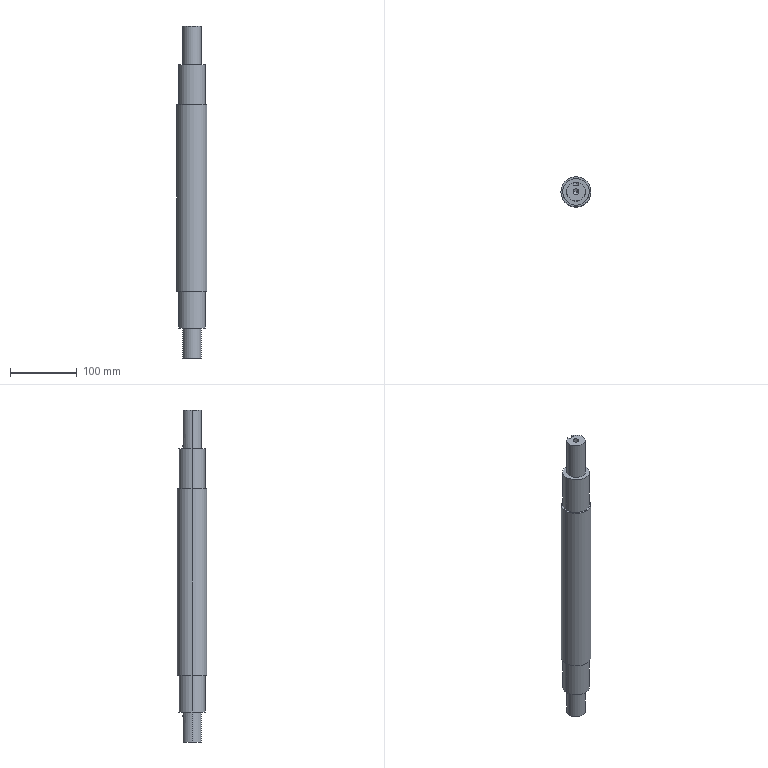Part | STEP file | Produce dryer line heating fan-SIROCCOFAN-3KW-SHAFT | 1 solid | 34 faces | box 45 x 45 x 498 mm | volume 647195 mm3 | cylinder 18 | plane 12 | cone 4 | commonest cylinder face diameters 8 x4 8.5 x4 28 x4 40 x4 45 x2
STEP:
#1=CARTESIAN_POINT('',(4.25,0.,-352.5));
#2=VERTEX_POINT('',#1);
#3=CARTESIAN_POINT('',(-4.25,0.,-352.5));
#4=VERTEX_POINT('',#3);
#5=CARTESIAN_POINT('',(0.,0.,-352.5));
#6=DIRECTION('',(0.,0.,-1.));
#7=DIRECTION('',(-1.,0.,0.));
#8=AXIS2_PLACEMENT_3D('',#5,#6,#7);
#9=CIRCLE('',#8,4.25);
#10=EDGE_CURVE('',#2,#4,#9,.T.);
#11=ORIENTED_EDGE('',*,*,#10,.F.);
#12=CARTESIAN_POINT('',(4.25,0.,-380.));
#13=VERTEX_POINT('',#12);
#14=CARTESIAN_POINT('',(4.25,0.,-380.));
#15=DIRECTION('',(0.,0.,-1.));
#16=VECTOR('',#15,1000.);
#17=LINE('',#14,#16);
#18=EDGE_CURVE('',#2,#13,#17,.T.);
#19=ORIENTED_EDGE('',*,*,#18,.T.);
#20=CARTESIAN_POINT('',(-4.25,0.,-380.));
#21=VERTEX_POINT('',#20);
#22=CARTESIAN_POINT('',(0.,0.,-380.));
#23=DIRECTION('',(0.,0.,-1.));
#24=DIRECTION('',(-1.,0.,0.));
#25=AXIS2_PLACEMENT_3D('',#22,#23,#24);
#26=CIRCLE('',#25,4.25);
#27=EDGE_CURVE('',#13,#21,#26,.T.);
#28=ORIENTED_EDGE('',*,*,#27,.T.);
#29=CARTESIAN_POINT('',(-4.25,0.,-380.));
#30=DIRECTION('',(0.,0.,-1.));
#31=VECTOR('',#30,1000.);
#32=LINE('',#29,#31);
#33=EDGE_CURVE('',#4,#21,#32,.T.);
#34=ORIENTED_EDGE('',*,*,#33,.F.);
#35=EDGE_LOOP('',(#11,#19,#28,#34));
#36=FACE_OUTER_BOUND('',#35,.T.);
#37=CARTESIAN_POINT('',(0.,0.,-380.));
#38=DIRECTION('',(0.,0.,-1.));
#39=DIRECTION('',(-1.,0.,0.));
#40=AXIS2_PLACEMENT_3D('',#37,#38,#39);
#41=CYLINDRICAL_SURFACE('',#40,4.25);
#42=ADVANCED_FACE('',(#36),#41,.F.);
#43=CARTESIAN_POINT('',(0.,0.,-349.946));
#44=VERTEX_POINT('',#43);
#45=CARTESIAN_POINT('',(-4.25,0.,-352.5));
#46=DIRECTION('',(-0.8572,0.,-0.515));
#47=VECTOR('',#46,1000.);
#48=LINE('',#45,#47);
#49=EDGE_CURVE('',#44,#4,#48,.T.);
#50=ORIENTED_EDGE('',*,*,#49,.F.);
#51=CARTESIAN_POINT('',(4.25,0.,-352.5));
#52=DIRECTION('',(0.8572,0.,-0.515));
#53=VECTOR('',#52,1000.);
#54=LINE('',#51,#53);
#55=EDGE_CURVE('',#44,#2,#54,.T.);
#56=ORIENTED_EDGE('',*,*,#55,.T.);
#57=ORIENTED_EDGE('',*,*,#10,.T.);
#58=EDGE_LOOP('',(#50,#56,#57));
#59=FACE_OUTER_BOUND('',#58,.T.);
#60=CARTESIAN_POINT('',(0.,0.,-352.5));
#61=DIRECTION('',(0.,0.,-1.));
#62=DIRECTION('',(-1.,0.,0.));
#63=AXIS2_PLACEMENT_3D('',#60,#61,#62);
#64=CONICAL_SURFACE('',#63,4.25,1.03);
#65=ADVANCED_FACE('',(#59),#64,.F.);
#66=CARTESIAN_POINT('',(-14.,0.,-380.));
#67=VERTEX_POINT('',#66);
#68=CARTESIAN_POINT('',(-4.,13.416,-380.));
#69=VERTEX_POINT('',#68);
#70=CARTESIAN_POINT('',(0.,0.,-380.));
#71=DIRECTION('',(0.,0.,-1.));
#72=DIRECTION('',(-1.,0.,0.));
#73=AXIS2_PLACEMENT_3D('',#70,#71,#72);
#74=CIRCLE('',#73,14.);
#75=EDGE_CURVE('',#67,#69,#74,.T.);
#76=ORIENTED_EDGE('',*,*,#75,.F.);
#77=CARTESIAN_POINT('',(-14.,0.,-335.));
#78=VERTEX_POINT('',#77);
#79=CARTESIAN_POINT('',(-14.,0.,-380.));
#80=DIRECTION('',(0.,0.,1.));
#81=VECTOR('',#80,1000.);
#82=LINE('',#79,#81);
#83=EDGE_CURVE('',#67,#78,#82,.T.);
#84=ORIENTED_EDGE('',*,*,#83,.T.);
#85=CARTESIAN_POINT('',(14.,0.,-335.));
#86=VERTEX_POINT('',#85);
#87=CARTESIAN_POINT('',(0.,0.,-335.));
#88=DIRECTION('',(0.,0.,-1.));
#89=DIRECTION('',(-1.,0.,0.));
#90=AXIS2_PLACEMENT_3D('',#87,#88,#89);
#91=CIRCLE('',#90,14.);
#92=EDGE_CURVE('',#78,#86,#91,.T.);
#93=ORIENTED_EDGE('',*,*,#92,.T.);
#94=CARTESIAN_POINT('',(14.,0.,-380.));
#95=VERTEX_POINT('',#94);
#96=CARTESIAN_POINT('',(14.,0.,-380.));
#97=DIRECTION('',(0.,0.,1.));
#98=VECTOR('',#97,1000.);
#99=LINE('',#96,#98);
#100=EDGE_CURVE('',#95,#86,#99,.T.);
#101=ORIENTED_EDGE('',*,*,#100,.F.);
#102=CARTESIAN_POINT('',(4.,13.416,-380.));
#103=VERTEX_POINT('',#102);
#104=CARTESIAN_POINT('',(0.,0.,-380.));
#105=DIRECTION('',(0.,0.,-1.));
#106=DIRECTION('',(-1.,0.,0.));
#107=AXIS2_PLACEMENT_3D('',#104,#105,#106);
#108=CIRCLE('',#107,14.);
#109=EDGE_CURVE('',#103,#95,#108,.T.);
#110=ORIENTED_EDGE('',*,*,#109,.F.);
#111=CARTESIAN_POINT('',(4.,13.416,-344.));
#112=VERTEX_POINT('',#111);
#113=CARTESIAN_POINT('',(4.,13.416,-380.));
#114=DIRECTION('',(0.,0.,1.));
#115=VECTOR('',#114,1000.);
#116=LINE('',#113,#115);
#117=EDGE_CURVE('',#103,#112,#116,.T.);
#118=ORIENTED_EDGE('',*,*,#117,.T.);
#119=CARTESIAN_POINT('',(0.,14.,-340.));
#120=VERTEX_POINT('',#119);
#121=CARTESIAN_POINT('',(4.,13.416,-344.));
#122=CARTESIAN_POINT('',(4.,13.416,-343.734));
#123=CARTESIAN_POINT('',(3.974,13.424,-343.474));
#124=CARTESIAN_POINT('',(3.871,13.454,-342.961));
#125=CARTESIAN_POINT('',(3.794,13.477,-342.706));
#126=CARTESIAN_POINT('',(3.593,13.531,-342.223));
#127=CARTESIAN_POINT('',(3.47,13.564,-341.994));
#128=CARTESIAN_POINT('',(3.18,13.635,-341.56));
#129=CARTESIAN_POINT('',(3.013,13.673,-341.356));
#130=CARTESIAN_POINT('',(2.646,13.749,-340.989));
#131=CARTESIAN_POINT('',(2.446,13.786,-340.824));
#132=CARTESIAN_POINT('',(2.009,13.857,-340.531));
#133=CARTESIAN_POINT('',(1.779,13.889,-340.408));
#134=CARTESIAN_POINT('',(1.299,13.942,-340.208));
#135=CARTESIAN_POINT('',(1.046,13.963,-340.13));
#136=CARTESIAN_POINT('',(0.5278,13.992,-340.026));
#137=CARTESIAN_POINT('',(0.2656,14.,-340.));
#138=CARTESIAN_POINT('',(0.,14.,-340.));
#139=B_SPLINE_CURVE_WITH_KNOTS('',3,(#121,#122,#123,#124,#125,#126,#127,#128,#129,#130,#131,#132,#133,#134,#135,#136,#137,#138),.UNSPECIFIED.,.F.,.F.,(4,2,2,2,2,2,2,2,4),(0.,0.0007852,0.00157,0.002356,0.003141,0.003926,0.004711,0.005496,0.006282),.UNSPECIFIED.);
#140=EDGE_CURVE('',#112,#120,#139,.T.);
#141=ORIENTED_EDGE('',*,*,#140,.T.);
#142=CARTESIAN_POINT('',(-4.,13.416,-344.));
#143=VERTEX_POINT('',#142);
#144=CARTESIAN_POINT('',(0.,14.,-340.));
#145=CARTESIAN_POINT('',(-0.2656,14.,-340.));
#146=CARTESIAN_POINT('',(-0.5265,13.992,-340.026));
#147=CARTESIAN_POINT('',(-1.039,13.964,-340.129));
#148=CARTESIAN_POINT('',(-1.294,13.942,-340.206));
#149=CARTESIAN_POINT('',(-1.778,13.889,-340.407));
#150=CARTESIAN_POINT('',(-2.007,13.857,-340.53));
#151=CARTESIAN_POINT('',(-2.44,13.787,-340.82));
#152=CARTESIAN_POINT('',(-2.645,13.749,-340.988));
#153=CARTESIAN_POINT('',(-3.011,13.674,-341.354));
#154=CARTESIAN_POINT('',(-3.176,13.636,-341.555));
#155=CARTESIAN_POINT('',(-3.469,13.564,-341.991));
#156=CARTESIAN_POINT('',(-3.592,13.532,-342.221));
#157=CARTESIAN_POINT('',(-3.792,13.477,-342.702));
#158=CARTESIAN_POINT('',(-3.87,13.455,-342.954));
#159=CARTESIAN_POINT('',(-3.974,13.424,-343.472));
#160=CARTESIAN_POINT('',(-4.,13.416,-343.734));
#161=CARTESIAN_POINT('',(-4.,13.416,-344.));
#162=B_SPLINE_CURVE_WITH_KNOTS('',3,(#144,#145,#146,#147,#148,#149,#150,#151,#152,#153,#154,#155,#156,#157,#158,#159,#160,#161),.UNSPECIFIED.,.F.,.F.,(4,2,2,2,2,2,2,2,4),(0.,0.0007852,0.00157,0.002356,0.003141,0.003926,0.004711,0.005496,0.006282),.UNSPECIFIED.);
#163=EDGE_CURVE('',#120,#143,#162,.T.);
#164=ORIENTED_EDGE('',*,*,#163,.T.);
#165=CARTESIAN_POINT('',(-4.,13.416,-380.));
#166=DIRECTION('',(0.,0.,-1.));
#167=VECTOR('',#166,1000.);
#168=LINE('',#165,#167);
#169=EDGE_CURVE('',#143,#69,#168,.T.);
#170=ORIENTED_EDGE('',*,*,#169,.T.);
#171=EDGE_LOOP('',(#76,#84,#93,#101,#110,#118,#141,#164,#170));
#172=FACE_OUTER_BOUND('',#171,.T.);
#173=CARTESIAN_POINT('',(0.,0.,-380.));
#174=DIRECTION('',(0.,0.,1.));
#175=DIRECTION('',(1.,0.,0.));
#176=AXIS2_PLACEMENT_3D('',#173,#174,#175);
#177=CYLINDRICAL_SURFACE('',#176,14.);
#178=ADVANCED_FACE('',(#172),#177,.T.);
#179=CARTESIAN_POINT('',(-20.,0.,-335.));
#180=VERTEX_POINT('',#179);
#181=CARTESIAN_POINT('',(20.,0.,-335.));
#182=VERTEX_POINT('',#181);
#183=CARTESIAN_POINT('',(0.,0.,-335.));
#184=DIRECTION('',(0.,0.,-1.));
#185=DIRECTION('',(-1.,0.,0.));
#186=AXIS2_PLACEMENT_3D('',#183,#184,#185);
#187=CIRCLE('',#186,20.);
#188=EDGE_CURVE('',#180,#182,#187,.T.);
#189=ORIENTED_EDGE('',*,*,#188,.F.);
#190=CARTESIAN_POINT('',(-20.,0.,-280.));
#191=VERTEX_POINT('',#190);
#192=CARTESIAN_POINT('',(-20.,0.,-335.));
#193=DIRECTION('',(0.,0.,1.));
#194=VECTOR('',#193,1000.);
#195=LINE('',#192,#194);
#196=EDGE_CURVE('',#180,#191,#195,.T.);
#197=ORIENTED_EDGE('',*,*,#196,.T.);
#198=CARTESIAN_POINT('',(20.,0.,-280.));
#199=VERTEX_POINT('',#198);
#200=CARTESIAN_POINT('',(0.,0.,-280.));
#201=DIRECTION('',(0.,0.,-1.));
#202=DIRECTION('',(-1.,0.,0.));
#203=AXIS2_PLACEMENT_3D('',#200,#201,#202);
#204=CIRCLE('',#203,20.);
#205=EDGE_CURVE('',#191,#199,#204,.T.);
#206=ORIENTED_EDGE('',*,*,#205,.T.);
#207=CARTESIAN_POINT('',(20.,0.,-335.));
#208=DIRECTION('',(0.,0.,1.));
#209=VECTOR('',#208,1000.);
#210=LINE('',#207,#209);
#211=EDGE_CURVE('',#182,#199,#210,.T.);
#212=ORIENTED_EDGE('',*,*,#211,.F.);
#213=EDGE_LOOP('',(#189,#197,#206,#212));
#214=FACE_OUTER_BOUND('',#213,.T.);
#215=CARTESIAN_POINT('',(0.,0.,-335.));
#216=DIRECTION('',(0.,0.,1.));
#217=DIRECTION('',(1.,0.,0.));
#218=AXIS2_PLACEMENT_3D('',#215,#216,#217);
#219=CYLINDRICAL_SURFACE('',#218,20.);
#220=ADVANCED_FACE('',(#214),#219,.T.);
#221=CARTESIAN_POINT('',(-4.25,0.,90.5));
#222=VERTEX_POINT('',#221);
#223=CARTESIAN_POINT('',(4.25,0.,90.5));
#224=VERTEX_POINT('',#223);
#225=CARTESIAN_POINT('',(0.,0.,90.5));
#226=DIRECTION('',(0.,0.,1.));
#227=DIRECTION('',(1.,0.,0.));
#228=AXIS2_PLACEMENT_3D('',#225,#226,#227);
#229=CIRCLE('',#228,4.25);
#230=EDGE_CURVE('',#222,#224,#229,.T.);
#231=ORIENTED_EDGE('',*,*,#230,.F.);
#232=CARTESIAN_POINT('',(-4.25,0.,118.));
#233=VERTEX_POINT('',#232);
#234=CARTESIAN_POINT('',(-4.25,0.,118.));
#235=DIRECTION('',(0.,0.,1.));
#236=VECTOR('',#235,1000.);
#237=LINE('',#234,#236);
#238=EDGE_CURVE('',#222,#233,#237,.T.);
#239=ORIENTED_EDGE('',*,*,#238,.T.);
#240=CARTESIAN_POINT('',(4.25,0.,118.));
#241=VERTEX_POINT('',#240);
#242=CARTESIAN_POINT('',(0.,0.,118.));
#243=DIRECTION('',(0.,0.,1.));
#244=DIRECTION('',(1.,0.,0.));
#245=AXIS2_PLACEMENT_3D('',#242,#243,#244);
#246=CIRCLE('',#245,4.25);
#247=EDGE_CURVE('',#233,#241,#246,.T.);
#248=ORIENTED_EDGE('',*,*,#247,.T.);
#249=CARTESIAN_POINT('',(4.25,0.,118.));
#250=DIRECTION('',(0.,0.,1.));
#251=VECTOR('',#250,1000.);
#252=LINE('',#249,#251);
#253=EDGE_CURVE('',#224,#241,#252,.T.);
#254=ORIENTED_EDGE('',*,*,#253,.F.);
#255=EDGE_LOOP('',(#231,#239,#248,#254));
#256=FACE_OUTER_BOUND('',#255,.T.);
#257=CARTESIAN_POINT('',(0.,0.,118.));
#258=DIRECTION('',(0.,0.,1.));
#259=DIRECTION('',(1.,0.,0.));
#260=AXIS2_PLACEMENT_3D('',#257,#258,#259);
#261=CYLINDRICAL_SURFACE('',#260,4.25);
#262=ADVANCED_FACE('',(#256),#261,.F.);
#263=CARTESIAN_POINT('',(0.,0.,87.946));
#264=VERTEX_POINT('',#263);
#265=CARTESIAN_POINT('',(4.25,0.,90.5));
#266=DIRECTION('',(0.8572,0.,0.515));
#267=VECTOR('',#266,1000.);
#268=LINE('',#265,#267);
#269=EDGE_CURVE('',#264,#224,#268,.T.);
#270=ORIENTED_EDGE('',*,*,#269,.F.);
#271=CARTESIAN_POINT('',(-4.25,0.,90.5));
#272=DIRECTION('',(-0.8572,0.,0.515));
#273=VECTOR('',#272,1000.);
#274=LINE('',#271,#273);
#275=EDGE_CURVE('',#264,#222,#274,.T.);
#276=ORIENTED_EDGE('',*,*,#275,.T.);
#277=ORIENTED_EDGE('',*,*,#230,.T.);
#278=EDGE_LOOP('',(#270,#276,#277));
#279=FACE_OUTER_BOUND('',#278,.T.);
#280=CARTESIAN_POINT('',(0.,0.,90.5));
#281=DIRECTION('',(0.,0.,1.));
#282=DIRECTION('',(1.,0.,0.));
#283=AXIS2_PLACEMENT_3D('',#280,#281,#282);
#284=CONICAL_SURFACE('',#283,4.25,1.03);
#285=ADVANCED_FACE('',(#279),#284,.F.);
#286=CARTESIAN_POINT('',(-22.5,0.,-280.));
#287=VERTEX_POINT('',#286);
#288=CARTESIAN_POINT('',(22.5,0.,-280.));
#289=VERTEX_POINT('',#288);
#290=CARTESIAN_POINT('',(0.,0.,-280.));
#291=DIRECTION('',(0.,0.,-1.));
#292=DIRECTION('',(-1.,0.,0.));
#293=AXIS2_PLACEMENT_3D('',#290,#291,#292);
#294=CIRCLE('',#293,22.5);
#295=EDGE_CURVE('',#287,#289,#294,.T.);
#296=ORIENTED_EDGE('',*,*,#295,.F.);
#297=CARTESIAN_POINT('',(-22.5,0.,0.));
#298=VERTEX_POINT('',#297);
#299=CARTESIAN_POINT('',(-22.5,0.,-280.));
#300=DIRECTION('',(0.,0.,1.));
#301=VECTOR('',#300,1000.);
#302=LINE('',#299,#301);
#303=EDGE_CURVE('',#287,#298,#302,.T.);
#304=ORIENTED_EDGE('',*,*,#303,.T.);
#305=CARTESIAN_POINT('',(22.5,0.,0.));
#306=VERTEX_POINT('',#305);
#307=CARTESIAN_POINT('',(0.,0.,0.));
#308=DIRECTION('',(0.,0.,-1.));
#309=DIRECTION('',(-1.,0.,0.));
#310=AXIS2_PLACEMENT_3D('',#307,#308,#309);
#311=CIRCLE('',#310,22.5);
#312=EDGE_CURVE('',#298,#306,#311,.T.);
#313=ORIENTED_EDGE('',*,*,#312,.T.);
#314=CARTESIAN_POINT('',(22.5,0.,-280.));
#315=DIRECTION('',(0.,0.,1.));
#316=VECTOR('',#315,1000.);
#317=LINE('',#314,#316);
#318=EDGE_CURVE('',#289,#306,#317,.T.);
#319=ORIENTED_EDGE('',*,*,#318,.F.);
#320=EDGE_LOOP('',(#296,#304,#313,#319));
#321=FACE_OUTER_BOUND('',#320,.T.);
#322=CARTESIAN_POINT('',(0.,0.,-280.));
#323=DIRECTION('',(0.,0.,1.));
#324=DIRECTION('',(1.,0.,0.));
#325=AXIS2_PLACEMENT_3D('',#322,#323,#324);
#326=CYLINDRICAL_SURFACE('',#325,22.5);
#327=ADVANCED_FACE('',(#321),#326,.T.);
#328=CARTESIAN_POINT('',(14.,0.,118.));
#329=VERTEX_POINT('',#328);
#330=CARTESIAN_POINT('',(4.,13.416,118.));
#331=VERTEX_POINT('',#330);
#332=CARTESIAN_POINT('',(0.,0.,118.));
#333=DIRECTION('',(0.,0.,1.));
#334=DIRECTION('',(1.,0.,0.));
#335=AXIS2_PLACEMENT_3D('',#332,#333,#334);
#336=CIRCLE('',#335,14.);
#337=EDGE_CURVE('',#329,#331,#336,.T.);
#338=ORIENTED_EDGE('',*,*,#337,.F.);
#339=CARTESIAN_POINT('',(14.,0.,60.));
#340=VERTEX_POINT('',#339);
#341=CARTESIAN_POINT('',(14.,0.,118.));
#342=DIRECTION('',(0.,0.,-1.));
#343=VECTOR('',#342,1000.);
#344=LINE('',#341,#343);
#345=EDGE_CURVE('',#329,#340,#344,.T.);
#346=ORIENTED_EDGE('',*,*,#345,.T.);
#347=CARTESIAN_POINT('',(-14.,0.,60.));
#348=VERTEX_POINT('',#347);
#349=CARTESIAN_POINT('',(0.,0.,60.));
#350=DIRECTION('',(0.,0.,1.));
#351=DIRECTION('',(1.,0.,0.));
#352=AXIS2_PLACEMENT_3D('',#349,#350,#351);
#353=CIRCLE('',#352,14.);
#354=EDGE_CURVE('',#340,#348,#353,.T.);
#355=ORIENTED_EDGE('',*,*,#354,.T.);
#356=CARTESIAN_POINT('',(-14.,0.,118.));
#357=VERTEX_POINT('',#356);
#358=CARTESIAN_POINT('',(-14.,0.,118.));
#359=DIRECTION('',(0.,0.,-1.));
#360=VECTOR('',#359,1000.);
#361=LINE('',#358,#360);
#362=EDGE_CURVE('',#357,#348,#361,.T.);
#363=ORIENTED_EDGE('',*,*,#362,.F.);
#364=CARTESIAN_POINT('',(-4.,13.416,118.));
#365=VERTEX_POINT('',#364);
#366=CARTESIAN_POINT('',(0.,0.,118.));
#367=DIRECTION('',(0.,0.,1.));
#368=DIRECTION('',(1.,0.,0.));
#369=AXIS2_PLACEMENT_3D('',#366,#367,#368);
#370=CIRCLE('',#369,14.);
#371=EDGE_CURVE('',#365,#357,#370,.T.);
#372=ORIENTED_EDGE('',*,*,#371,.F.);
#373=CARTESIAN_POINT('',(-4.,13.416,67.));
#374=VERTEX_POINT('',#373);
#375=CARTESIAN_POINT('',(-4.,13.416,118.));
#376=DIRECTION('',(0.,0.,-1.));
#377=VECTOR('',#376,1000.);
#378=LINE('',#375,#377);
#379=EDGE_CURVE('',#365,#374,#378,.T.);
#380=ORIENTED_EDGE('',*,*,#379,.T.);
#381=CARTESIAN_POINT('',(0.,14.,63.));
#382=VERTEX_POINT('',#381);
#383=CARTESIAN_POINT('',(-4.,13.416,67.));
#384=CARTESIAN_POINT('',(-4.,13.416,66.734));
#385=CARTESIAN_POINT('',(-3.974,13.424,66.474));
#386=CARTESIAN_POINT('',(-3.871,13.454,65.961));
#387=CARTESIAN_POINT('',(-3.794,13.477,65.706));
#388=CARTESIAN_POINT('',(-3.593,13.531,65.223));
#389=CARTESIAN_POINT('',(-3.47,13.564,64.994));
#390=CARTESIAN_POINT('',(-3.18,13.635,64.56));
#391=CARTESIAN_POINT('',(-3.013,13.673,64.356));
#392=CARTESIAN_POINT('',(-2.646,13.749,63.989));
#393=CARTESIAN_POINT('',(-2.446,13.786,63.824));
#394=CARTESIAN_POINT('',(-2.009,13.857,63.531));
#395=CARTESIAN_POINT('',(-1.779,13.889,63.408));
#396=CARTESIAN_POINT('',(-1.299,13.942,63.208));
#397=CARTESIAN_POINT('',(-1.046,13.963,63.13));
#398=CARTESIAN_POINT('',(-0.5278,13.992,63.026));
#399=CARTESIAN_POINT('',(-0.2656,14.,63.));
#400=CARTESIAN_POINT('',(0.,14.,63.));
#401=B_SPLINE_CURVE_WITH_KNOTS('',3,(#383,#384,#385,#386,#387,#388,#389,#390,#391,#392,#393,#394,#395,#396,#397,#398,#399,#400),.UNSPECIFIED.,.F.,.F.,(4,2,2,2,2,2,2,2,4),(0.,0.0007852,0.00157,0.002356,0.003141,0.003926,0.004711,0.005496,0.006282),.UNSPECIFIED.);
#402=EDGE_CURVE('',#374,#382,#401,.T.);
#403=ORIENTED_EDGE('',*,*,#402,.T.);
#404=CARTESIAN_POINT('',(4.,13.416,67.));
#405=VERTEX_POINT('',#404);
#406=CARTESIAN_POINT('',(0.,14.,63.));
#407=CARTESIAN_POINT('',(0.2656,14.,63.));
#408=CARTESIAN_POINT('',(0.5265,13.992,63.026));
#409=CARTESIAN_POINT('',(1.039,13.964,63.129));
#410=CARTESIAN_POINT('',(1.294,13.942,63.206));
#411=CARTESIAN_POINT('',(1.778,13.889,63.407));
#412=CARTESIAN_POINT('',(2.007,13.857,63.53));
#413=CARTESIAN_POINT('',(2.44,13.787,63.82));
#414=CARTESIAN_POINT('',(2.645,13.749,63.988));
#415=CARTESIAN_POINT('',(3.011,13.674,64.354));
#416=CARTESIAN_POINT('',(3.176,13.636,64.555));
#417=CARTESIAN_POINT('',(3.469,13.564,64.991));
#418=CARTESIAN_POINT('',(3.592,13.532,65.221));
#419=CARTESIAN_POINT('',(3.792,13.477,65.702));
#420=CARTESIAN_POINT('',(3.87,13.455,65.954));
#421=CARTESIAN_POINT('',(3.974,13.424,66.472));
#422=CARTESIAN_POINT('',(4.,13.416,66.734));
#423=CARTESIAN_POINT('',(4.,13.416,67.));
#424=B_SPLINE_CURVE_WITH_KNOTS('',3,(#406,#407,#408,#409,#410,#411,#412,#413,#414,#415,#416,#417,#418,#419,#420,#421,#422,#423),.UNSPECIFIED.,.F.,.F.,(4,2,2,2,2,2,2,2,4),(0.,0.0007852,0.00157,0.002356,0.003141,0.003926,0.004711,0.005496,0.006282),.UNSPECIFIED.);
#425=EDGE_CURVE('',#382,#405,#424,.T.);
#426=ORIENTED_EDGE('',*,*,#425,.T.);
#427=CARTESIAN_POINT('',(4.,13.416,118.));
#428=DIRECTION('',(0.,0.,1.));
#429=VECTOR('',#428,1000.);
#430=LINE('',#427,#429);
#431=EDGE_CURVE('',#405,#331,#430,.T.);
#432=ORIENTED_EDGE('',*,*,#431,.T.);
#433=EDGE_LOOP('',(#338,#346,#355,#363,#372,#380,#403,#426,#432));
#434=FACE_OUTER_BOUND('',#433,.T.);
#435=CARTESIAN_POINT('',(0.,0.,118.));
#436=DIRECTION('',(0.,0.,-1.));
#437=DIRECTION('',(-1.,0.,0.));
#438=AXIS2_PLACEMENT_3D('',#435,#436,#437);
#439=CYLINDRICAL_SURFACE('',#438,14.);
#440=ADVANCED_FACE('',(#434),#439,.T.);
#441=CARTESIAN_POINT('',(20.,0.,60.));
#442=VERTEX_POINT('',#441);
#443=CARTESIAN_POINT('',(-20.,0.,60.));
#444=VERTEX_POINT('',#443);
#445=CARTESIAN_POINT('',(0.,0.,60.));
#446=DIRECTION('',(0.,0.,1.));
#447=DIRECTION('',(1.,0.,0.));
#448=AXIS2_PLACEMENT_3D('',#445,#446,#447);
#449=CIRCLE('',#448,20.);
#450=EDGE_CURVE('',#442,#444,#449,.T.);
#451=ORIENTED_EDGE('',*,*,#450,.F.);
#452=CARTESIAN_POINT('',(20.,0.,0.));
#453=VERTEX_POINT('',#452);
#454=CARTESIAN_POINT('',(20.,0.,60.));
#455=DIRECTION('',(0.,0.,-1.));
#456=VECTOR('',#455,1000.);
#457=LINE('',#454,#456);
#458=EDGE_CURVE('',#442,#453,#457,.T.);
#459=ORIENTED_EDGE('',*,*,#458,.T.);
#460=CARTESIAN_POINT('',(-20.,0.,0.));
#461=VERTEX_POINT('',#460);
#462=CARTESIAN_POINT('',(0.,0.,0.));
#463=DIRECTION('',(0.,0.,-1.));
#464=DIRECTION('',(-1.,0.,0.));
#465=AXIS2_PLACEMENT_3D('',#462,#463,#464);
#466=CIRCLE('',#465,20.);
#467=EDGE_CURVE('',#461,#453,#466,.T.);
#468=ORIENTED_EDGE('',*,*,#467,.F.);
#469=CARTESIAN_POINT('',(-20.,0.,60.));
#470=DIRECTION('',(0.,0.,-1.));
#471=VECTOR('',#470,1000.);
#472=LINE('',#469,#471);
#473=EDGE_CURVE('',#444,#461,#472,.T.);
#474=ORIENTED_EDGE('',*,*,#473,.F.);
#475=EDGE_LOOP('',(#451,#459,#468,#474));
#476=FACE_OUTER_BOUND('',#475,.T.);
#477=CARTESIAN_POINT('',(0.,0.,60.));
#478=DIRECTION('',(0.,0.,-1.));
#479=DIRECTION('',(-1.,0.,0.));
#480=AXIS2_PLACEMENT_3D('',#477,#478,#479);
#481=CYLINDRICAL_SURFACE('',#480,20.);
#482=ADVANCED_FACE('',(#476),#481,.T.);
#483=CARTESIAN_POINT('',(0.,0.,-335.));
#484=DIRECTION('',(0.,0.,-1.));
#485=DIRECTION('',(-1.,0.,0.));
#486=AXIS2_PLACEMENT_3D('',#483,#484,#485);
#487=CIRCLE('',#486,20.);
#488=EDGE_CURVE('',#182,#180,#487,.T.);
#489=ORIENTED_EDGE('',*,*,#488,.T.);
#490=ORIENTED_EDGE('',*,*,#188,.T.);
#491=EDGE_LOOP('',(#489,#490));
#492=FACE_OUTER_BOUND('',#491,.T.);
#493=CARTESIAN_POINT('',(0.,0.,-335.));
#494=DIRECTION('',(0.,0.,-1.));
#495=DIRECTION('',(-1.,0.,0.));
#496=AXIS2_PLACEMENT_3D('',#493,#494,#495);
#497=CIRCLE('',#496,14.);
#498=EDGE_CURVE('',#86,#78,#497,.T.);
#499=ORIENTED_EDGE('',*,*,#498,.F.);
#500=ORIENTED_EDGE('',*,*,#92,.F.);
#501=EDGE_LOOP('',(#499,#500));
#502=FACE_BOUND('',#501,.T.);
#503=CARTESIAN_POINT('',(0.,0.,-335.));
#504=DIRECTION('',(0.,0.,-1.));
#505=DIRECTION('',(-1.,0.,0.));
#506=AXIS2_PLACEMENT_3D('',#503,#504,#505);
#507=PLANE('',#506);
#508=ADVANCED_FACE('',(#492,#502),#507,.T.);
#509=CARTESIAN_POINT('',(0.,0.,-280.));
#510=DIRECTION('',(0.,0.,-1.));
#511=DIRECTION('',(-1.,0.,0.));
#512=AXIS2_PLACEMENT_3D('',#509,#510,#511);
#513=CIRCLE('',#512,22.5);
#514=EDGE_CURVE('',#289,#287,#513,.T.);
#515=ORIENTED_EDGE('',*,*,#514,.T.);
#516=ORIENTED_EDGE('',*,*,#295,.T.);
#517=EDGE_LOOP('',(#515,#516));
#518=FACE_OUTER_BOUND('',#517,.T.);
#519=CARTESIAN_POINT('',(0.,0.,-280.));
#520=DIRECTION('',(0.,0.,-1.));
#521=DIRECTION('',(-1.,0.,0.));
#522=AXIS2_PLACEMENT_3D('',#519,#520,#521);
#523=CIRCLE('',#522,20.);
#524=EDGE_CURVE('',#199,#191,#523,.T.);
#525=ORIENTED_EDGE('',*,*,#524,.F.);
#526=ORIENTED_EDGE('',*,*,#205,.F.);
#527=EDGE_LOOP('',(#525,#526));
#528=FACE_BOUND('',#527,.T.);
#529=CARTESIAN_POINT('',(0.,0.,-280.));
#530=DIRECTION('',(0.,0.,-1.));
#531=DIRECTION('',(-1.,0.,0.));
#532=AXIS2_PLACEMENT_3D('',#529,#530,#531);
#533=PLANE('',#532);
#534=ADVANCED_FACE('',(#518,#528),#533,.T.);
#535=CARTESIAN_POINT('',(0.,0.,60.));
#536=DIRECTION('',(0.,0.,1.));
#537=DIRECTION('',(1.,0.,0.));
#538=AXIS2_PLACEMENT_3D('',#535,#536,#537);
#539=CIRCLE('',#538,20.);
#540=EDGE_CURVE('',#444,#442,#539,.T.);
#541=ORIENTED_EDGE('',*,*,#540,.T.);
#542=ORIENTED_EDGE('',*,*,#450,.T.);
#543=EDGE_LOOP('',(#541,#542));
#544=FACE_OUTER_BOUND('',#543,.T.);
#545=CARTESIAN_POINT('',(0.,0.,60.));
#546=DIRECTION('',(0.,0.,1.));
#547=DIRECTION('',(1.,0.,0.));
#548=AXIS2_PLACEMENT_3D('',#545,#546,#547);
#549=CIRCLE('',#548,14.);
#550=EDGE_CURVE('',#348,#340,#549,.T.);
#551=ORIENTED_EDGE('',*,*,#550,.F.);
#552=ORIENTED_EDGE('',*,*,#354,.F.);
#553=EDGE_LOOP('',(#551,#552));
#554=FACE_BOUND('',#553,.T.);
#555=CARTESIAN_POINT('',(0.,0.,60.));
#556=DIRECTION('',(0.,0.,1.));
#557=DIRECTION('',(1.,0.,0.));
#558=AXIS2_PLACEMENT_3D('',#555,#556,#557);
#559=PLANE('',#558);
#560=ADVANCED_FACE('',(#544,#554),#559,.T.);
#561=ORIENTED_EDGE('',*,*,#458,.F.);
#562=ORIENTED_EDGE('',*,*,#540,.F.);
#563=ORIENTED_EDGE('',*,*,#473,.T.);
#564=CARTESIAN_POINT('',(0.,0.,0.));
#565=DIRECTION('',(0.,0.,-1.));
#566=DIRECTION('',(-1.,0.,0.));
#567=AXIS2_PLACEMENT_3D('',#564,#565,#566);
#568=CIRCLE('',#567,20.);
#569=EDGE_CURVE('',#453,#461,#568,.T.);
#570=ORIENTED_EDGE('',*,*,#569,.F.);
#571=EDGE_LOOP('',(#561,#562,#563,#570));
#572=FACE_OUTER_BOUND('',#571,.T.);
#573=CARTESIAN_POINT('',(0.,0.,60.));
#574=DIRECTION('',(0.,0.,-1.));
#575=DIRECTION('',(-1.,0.,0.));
#576=AXIS2_PLACEMENT_3D('',#573,#574,#575);
#577=CYLINDRICAL_SURFACE('',#576,20.);
#578=ADVANCED_FACE('',(#572),#577,.T.);
#579=ORIENTED_EDGE('',*,*,#345,.F.);
#580=CARTESIAN_POINT('',(0.,0.,118.));
#581=DIRECTION('',(0.,0.,1.));
#582=DIRECTION('',(1.,0.,0.));
#583=AXIS2_PLACEMENT_3D('',#580,#581,#582);
#584=CIRCLE('',#583,14.);
#585=EDGE_CURVE('',#357,#329,#584,.T.);
#586=ORIENTED_EDGE('',*,*,#585,.F.);
#587=ORIENTED_EDGE('',*,*,#362,.T.);
#588=ORIENTED_EDGE('',*,*,#550,.T.);
#589=EDGE_LOOP('',(#579,#586,#587,#588));
#590=FACE_OUTER_BOUND('',#589,.T.);
#591=CARTESIAN_POINT('',(0.,0.,118.));
#592=DIRECTION('',(0.,0.,-1.));
#593=DIRECTION('',(-1.,0.,0.));
#594=AXIS2_PLACEMENT_3D('',#591,#592,#593);
#595=CYLINDRICAL_SURFACE('',#594,14.);
#596=ADVANCED_FACE('',(#590),#595,.T.);
#597=CARTESIAN_POINT('',(-4.,10.,118.));
#598=VERTEX_POINT('',#597);
#599=CARTESIAN_POINT('',(-4.,0.,118.));
#600=DIRECTION('',(0.,-1.,0.));
#601=VECTOR('',#600,1000.);
#602=LINE('',#599,#601);
#603=EDGE_CURVE('',#365,#598,#602,.T.);
#604=ORIENTED_EDGE('',*,*,#603,.F.);
#605=ORIENTED_EDGE('',*,*,#371,.T.);
#606=ORIENTED_EDGE('',*,*,#585,.T.);
#607=ORIENTED_EDGE('',*,*,#337,.T.);
#608=CARTESIAN_POINT('',(4.,10.,118.));
#609=VERTEX_POINT('',#608);
#610=CARTESIAN_POINT('',(4.,18.,118.));
#611=DIRECTION('',(0.,1.,0.));
#612=VECTOR('',#611,1000.);
#613=LINE('',#610,#612);
#614=EDGE_CURVE('',#609,#331,#613,.T.);
#615=ORIENTED_EDGE('',*,*,#614,.F.);
#616=CARTESIAN_POINT('',(-4.,10.,118.));
#617=DIRECTION('',(1.,0.,0.));
#618=VECTOR('',#617,1000.);
#619=LINE('',#616,#618);
#620=EDGE_CURVE('',#598,#609,#619,.T.);
#621=ORIENTED_EDGE('',*,*,#620,.F.);
#622=EDGE_LOOP('',(#604,#605,#606,#607,#615,#621));
#623=FACE_OUTER_BOUND('',#622,.T.);
#624=CARTESIAN_POINT('',(0.,0.,118.));
#625=DIRECTION('',(0.,0.,1.));
#626=DIRECTION('',(1.,0.,0.));
#627=AXIS2_PLACEMENT_3D('',#624,#625,#626);
#628=CIRCLE('',#627,4.25);
#629=EDGE_CURVE('',#241,#233,#628,.T.);
#630=ORIENTED_EDGE('',*,*,#629,.F.);
#631=ORIENTED_EDGE('',*,*,#247,.F.);
#632=EDGE_LOOP('',(#630,#631));
#633=FACE_BOUND('',#632,.T.);
#634=CARTESIAN_POINT('',(0.,0.,118.));
#635=DIRECTION('',(0.,0.,1.));
#636=DIRECTION('',(1.,0.,0.));
#637=AXIS2_PLACEMENT_3D('',#634,#635,#636);
#638=PLANE('',#637);
#639=ADVANCED_FACE('',(#623,#633),#638,.T.);
#640=CARTESIAN_POINT('',(0.,0.,0.));
#641=DIRECTION('',(0.,0.,-1.));
#642=DIRECTION('',(-1.,0.,0.));
#643=AXIS2_PLACEMENT_3D('',#640,#641,#642);
#644=CIRCLE('',#643,22.5);
#645=EDGE_CURVE('',#306,#298,#644,.T.);
#646=ORIENTED_EDGE('',*,*,#645,.F.);
#647=ORIENTED_EDGE('',*,*,#312,.F.);
#648=EDGE_LOOP('',(#646,#647));
#649=FACE_OUTER_BOUND('',#648,.T.);
#650=ORIENTED_EDGE('',*,*,#467,.T.);
#651=ORIENTED_EDGE('',*,*,#569,.T.);
#652=EDGE_LOOP('',(#650,#651));
#653=FACE_BOUND('',#652,.T.);
#654=CARTESIAN_POINT('',(0.,0.,0.));
#655=DIRECTION('',(0.,0.,-1.));
#656=DIRECTION('',(-1.,0.,0.));
#657=AXIS2_PLACEMENT_3D('',#654,#655,#656);
#658=PLANE('',#657);
#659=ADVANCED_FACE('',(#649,#653),#658,.F.);
#660=ORIENTED_EDGE('',*,*,#303,.F.);
#661=ORIENTED_EDGE('',*,*,#514,.F.);
#662=ORIENTED_EDGE('',*,*,#318,.T.);
#663=ORIENTED_EDGE('',*,*,#645,.T.);
#664=EDGE_LOOP('',(#660,#661,#662,#663));
#665=FACE_OUTER_BOUND('',#664,.T.);
#666=CARTESIAN_POINT('',(0.,0.,-280.));
#667=DIRECTION('',(0.,0.,1.));
#668=DIRECTION('',(1.,0.,0.));
#669=AXIS2_PLACEMENT_3D('',#666,#667,#668);
#670=CYLINDRICAL_SURFACE('',#669,22.5);
#671=ADVANCED_FACE('',(#665),#670,.T.);
#672=ORIENTED_EDGE('',*,*,#275,.F.);
#673=ORIENTED_EDGE('',*,*,#269,.T.);
#674=CARTESIAN_POINT('',(0.,0.,90.5));
#675=DIRECTION('',(0.,0.,1.));
#676=DIRECTION('',(1.,0.,0.));
#677=AXIS2_PLACEMENT_3D('',#674,#675,#676);
#678=CIRCLE('',#677,4.25);
#679=EDGE_CURVE('',#224,#222,#678,.T.);
#680=ORIENTED_EDGE('',*,*,#679,.T.);
#681=EDGE_LOOP('',(#672,#673,#680));
#682=FACE_OUTER_BOUND('',#681,.T.);
#683=CARTESIAN_POINT('',(0.,0.,90.5));
#684=DIRECTION('',(0.,0.,1.));
#685=DIRECTION('',(1.,0.,0.));
#686=AXIS2_PLACEMENT_3D('',#683,#684,#685);
#687=CONICAL_SURFACE('',#686,4.25,1.03);
#688=ADVANCED_FACE('',(#682),#687,.F.);
#689=ORIENTED_EDGE('',*,*,#238,.F.);
#690=ORIENTED_EDGE('',*,*,#679,.F.);
#691=ORIENTED_EDGE('',*,*,#253,.T.);
#692=ORIENTED_EDGE('',*,*,#629,.T.);
#693=EDGE_LOOP('',(#689,#690,#691,#692));
#694=FACE_OUTER_BOUND('',#693,.T.);
#695=CARTESIAN_POINT('',(0.,0.,118.));
#696=DIRECTION('',(0.,0.,1.));
#697=DIRECTION('',(1.,0.,0.));
#698=AXIS2_PLACEMENT_3D('',#695,#696,#697);
#699=CYLINDRICAL_SURFACE('',#698,4.25);
#700=ADVANCED_FACE('',(#694),#699,.F.);
#701=ORIENTED_EDGE('',*,*,#196,.F.);
#702=ORIENTED_EDGE('',*,*,#488,.F.);
#703=ORIENTED_EDGE('',*,*,#211,.T.);
#704=ORIENTED_EDGE('',*,*,#524,.T.);
#705=EDGE_LOOP('',(#701,#702,#703,#704));
#706=FACE_OUTER_BOUND('',#705,.T.);
#707=CARTESIAN_POINT('',(0.,0.,-335.));
#708=DIRECTION('',(0.,0.,1.));
#709=DIRECTION('',(1.,0.,0.));
#710=AXIS2_PLACEMENT_3D('',#707,#708,#709);
#711=CYLINDRICAL_SURFACE('',#710,20.);
#712=ADVANCED_FACE('',(#706),#711,.T.);
#713=ORIENTED_EDGE('',*,*,#83,.F.);
#714=CARTESIAN_POINT('',(0.,0.,-380.));
#715=DIRECTION('',(0.,0.,-1.));
#716=DIRECTION('',(-1.,0.,0.));
#717=AXIS2_PLACEMENT_3D('',#714,#715,#716);
#718=CIRCLE('',#717,14.);
#719=EDGE_CURVE('',#95,#67,#718,.T.);
#720=ORIENTED_EDGE('',*,*,#719,.F.);
#721=ORIENTED_EDGE('',*,*,#100,.T.);
#722=ORIENTED_EDGE('',*,*,#498,.T.);
#723=EDGE_LOOP('',(#713,#720,#721,#722));
#724=FACE_OUTER_BOUND('',#723,.T.);
#725=CARTESIAN_POINT('',(0.,0.,-380.));
#726=DIRECTION('',(0.,0.,1.));
#727=DIRECTION('',(1.,0.,0.));
#728=AXIS2_PLACEMENT_3D('',#725,#726,#727);
#729=CYLINDRICAL_SURFACE('',#728,14.);
#730=ADVANCED_FACE('',(#724),#729,.T.);
#731=CARTESIAN_POINT('',(0.,0.,-380.));
#732=DIRECTION('',(0.,0.,-1.));
#733=DIRECTION('',(-1.,0.,0.));
#734=AXIS2_PLACEMENT_3D('',#731,#732,#733);
#735=CIRCLE('',#734,4.25);
#736=EDGE_CURVE('',#21,#13,#735,.T.);
#737=ORIENTED_EDGE('',*,*,#736,.F.);
#738=ORIENTED_EDGE('',*,*,#27,.F.);
#739=EDGE_LOOP('',(#737,#738));
#740=FACE_BOUND('',#739,.T.);
#741=CARTESIAN_POINT('',(4.,10.,-380.));
#742=VERTEX_POINT('',#741);
#743=CARTESIAN_POINT('',(4.,0.,-380.));
#744=DIRECTION('',(0.,-1.,0.));
#745=VECTOR('',#744,1000.);
#746=LINE('',#743,#745);
#747=EDGE_CURVE('',#103,#742,#746,.T.);
#748=ORIENTED_EDGE('',*,*,#747,.F.);
#749=ORIENTED_EDGE('',*,*,#109,.T.);
#750=ORIENTED_EDGE('',*,*,#719,.T.);
#751=ORIENTED_EDGE('',*,*,#75,.T.);
#752=CARTESIAN_POINT('',(-4.,10.,-380.));
#753=VERTEX_POINT('',#752);
#754=CARTESIAN_POINT('',(-4.,16.,-380.));
#755=DIRECTION('',(0.,1.,0.));
#756=VECTOR('',#755,1000.);
#757=LINE('',#754,#756);
#758=EDGE_CURVE('',#753,#69,#757,.T.);
#759=ORIENTED_EDGE('',*,*,#758,.F.);
#760=CARTESIAN_POINT('',(4.,10.,-380.));
#761=DIRECTION('',(-1.,0.,0.));
#762=VECTOR('',#761,1000.);
#763=LINE('',#760,#762);
#764=EDGE_CURVE('',#742,#753,#763,.T.);
#765=ORIENTED_EDGE('',*,*,#764,.F.);
#766=EDGE_LOOP('',(#748,#749,#750,#751,#759,#765));
#767=FACE_OUTER_BOUND('',#766,.T.);
#768=CARTESIAN_POINT('',(0.,0.,-380.));
#769=DIRECTION('',(0.,0.,-1.));
#770=DIRECTION('',(-1.,0.,0.));
#771=AXIS2_PLACEMENT_3D('',#768,#769,#770);
#772=PLANE('',#771);
#773=ADVANCED_FACE('',(#740,#767),#772,.T.);
#774=CARTESIAN_POINT('',(-4.,10.,67.));
#775=VERTEX_POINT('',#774);
#776=CARTESIAN_POINT('',(-4.,10.,63.));
#777=DIRECTION('',(0.,0.,1.));
#778=VECTOR('',#777,1000.);
#779=LINE('',#776,#778);
#780=EDGE_CURVE('',#775,#598,#779,.T.);
#781=ORIENTED_EDGE('',*,*,#780,.F.);
#782=CARTESIAN_POINT('',(-4.,18.,67.));
#783=DIRECTION('',(0.,1.,0.));
#784=VECTOR('',#783,1000.);
#785=LINE('',#782,#784);
#786=EDGE_CURVE('',#775,#374,#785,.T.);
#787=ORIENTED_EDGE('',*,*,#786,.T.);
#788=ORIENTED_EDGE('',*,*,#379,.F.);
#789=ORIENTED_EDGE('',*,*,#603,.T.);
#790=EDGE_LOOP('',(#781,#787,#788,#789));
#791=FACE_OUTER_BOUND('',#790,.T.);
#792=CARTESIAN_POINT('',(-4.,18.,63.));
#793=DIRECTION('',(-1.,0.,0.));
#794=DIRECTION('',(0.,-1.,0.));
#795=AXIS2_PLACEMENT_3D('',#792,#793,#794);
#796=PLANE('',#795);
#797=ADVANCED_FACE('',(#791),#796,.F.);
#798=ORIENTED_EDGE('',*,*,#431,.F.);
#799=CARTESIAN_POINT('',(4.,10.,67.));
#800=VERTEX_POINT('',#799);
#801=CARTESIAN_POINT('',(4.,18.,67.));
#802=DIRECTION('',(0.,-1.,0.));
#803=VECTOR('',#802,1000.);
#804=LINE('',#801,#803);
#805=EDGE_CURVE('',#405,#800,#804,.T.);
#806=ORIENTED_EDGE('',*,*,#805,.T.);
#807=CARTESIAN_POINT('',(4.,10.,63.));
#808=DIRECTION('',(0.,0.,1.));
#809=VECTOR('',#808,1000.);
#810=LINE('',#807,#809);
#811=EDGE_CURVE('',#800,#609,#810,.T.);
#812=ORIENTED_EDGE('',*,*,#811,.T.);
#813=ORIENTED_EDGE('',*,*,#614,.T.);
#814=EDGE_LOOP('',(#798,#806,#812,#813));
#815=FACE_OUTER_BOUND('',#814,.T.);
#816=CARTESIAN_POINT('',(4.,18.,63.));
#817=DIRECTION('',(1.,0.,0.));
#818=DIRECTION('',(0.,1.,0.));
#819=AXIS2_PLACEMENT_3D('',#816,#817,#818);
#820=PLANE('',#819);
#821=ADVANCED_FACE('',(#815),#820,.F.);
#822=ORIENTED_EDGE('',*,*,#811,.F.);
#823=CARTESIAN_POINT('',(0.,10.,63.));
#824=VERTEX_POINT('',#823);
#825=CARTESIAN_POINT('',(0.,10.,67.));
#826=DIRECTION('',(0.,1.,0.));
#827=DIRECTION('',(1.,0.,0.));
#828=AXIS2_PLACEMENT_3D('',#825,#826,#827);
#829=CIRCLE('',#828,4.);
#830=EDGE_CURVE('',#800,#824,#829,.T.);
#831=ORIENTED_EDGE('',*,*,#830,.T.);
#832=CARTESIAN_POINT('',(0.,10.,67.));
#833=DIRECTION('',(0.,1.,0.));
#834=DIRECTION('',(1.,0.,0.));
#835=AXIS2_PLACEMENT_3D('',#832,#833,#834);
#836=CIRCLE('',#835,4.);
#837=EDGE_CURVE('',#824,#775,#836,.T.);
#838=ORIENTED_EDGE('',*,*,#837,.T.);
#839=ORIENTED_EDGE('',*,*,#780,.T.);
#840=ORIENTED_EDGE('',*,*,#620,.T.);
#841=EDGE_LOOP('',(#822,#831,#838,#839,#840));
#842=FACE_OUTER_BOUND('',#841,.T.);
#843=CARTESIAN_POINT('',(-4.,10.,63.));
#844=DIRECTION('',(0.,-1.,0.));
#845=DIRECTION('',(1.,0.,0.));
#846=AXIS2_PLACEMENT_3D('',#843,#844,#845);
#847=PLANE('',#846);
#848=ADVANCED_FACE('',(#842),#847,.F.);
#849=ORIENTED_EDGE('',*,*,#786,.F.);
#850=ORIENTED_EDGE('',*,*,#837,.F.);
#851=CARTESIAN_POINT('',(0.,10.,63.));
#852=DIRECTION('',(0.,-1.,0.));
#853=VECTOR('',#852,1000.);
#854=LINE('',#851,#853);
#855=EDGE_CURVE('',#382,#824,#854,.T.);
#856=ORIENTED_EDGE('',*,*,#855,.F.);
#857=ORIENTED_EDGE('',*,*,#402,.F.);
#858=EDGE_LOOP('',(#849,#850,#856,#857));
#859=FACE_OUTER_BOUND('',#858,.T.);
#860=CARTESIAN_POINT('',(0.,10.,67.));
#861=DIRECTION('',(0.,-1.,0.));
#862=DIRECTION('',(1.,0.,0.));
#863=AXIS2_PLACEMENT_3D('',#860,#861,#862);
#864=CYLINDRICAL_SURFACE('',#863,4.);
#865=ADVANCED_FACE('',(#859),#864,.F.);
#866=ORIENTED_EDGE('',*,*,#830,.F.);
#867=ORIENTED_EDGE('',*,*,#805,.F.);
#868=ORIENTED_EDGE('',*,*,#425,.F.);
#869=ORIENTED_EDGE('',*,*,#855,.T.);
#870=EDGE_LOOP('',(#866,#867,#868,#869));
#871=FACE_OUTER_BOUND('',#870,.T.);
#872=CARTESIAN_POINT('',(0.,10.,67.));
#873=DIRECTION('',(0.,1.,0.));
#874=DIRECTION('',(-1.,0.,0.));
#875=AXIS2_PLACEMENT_3D('',#872,#873,#874);
#876=CYLINDRICAL_SURFACE('',#875,4.);
#877=ADVANCED_FACE('',(#871),#876,.F.);
#878=CARTESIAN_POINT('',(4.,10.,-344.));
#879=VERTEX_POINT('',#878);
#880=CARTESIAN_POINT('',(4.,10.,-340.));
#881=DIRECTION('',(0.,0.,-1.));
#882=VECTOR('',#881,1000.);
#883=LINE('',#880,#882);
#884=EDGE_CURVE('',#879,#742,#883,.T.);
#885=ORIENTED_EDGE('',*,*,#884,.F.);
#886=CARTESIAN_POINT('',(4.,16.,-344.));
#887=DIRECTION('',(0.,1.,0.));
#888=VECTOR('',#887,1000.);
#889=LINE('',#886,#888);
#890=EDGE_CURVE('',#879,#112,#889,.T.);
#891=ORIENTED_EDGE('',*,*,#890,.T.);
#892=ORIENTED_EDGE('',*,*,#117,.F.);
#893=ORIENTED_EDGE('',*,*,#747,.T.);
#894=EDGE_LOOP('',(#885,#891,#892,#893));
#895=FACE_OUTER_BOUND('',#894,.T.);
#896=CARTESIAN_POINT('',(4.,16.,-340.));
#897=DIRECTION('',(1.,0.,0.));
#898=DIRECTION('',(0.,1.,0.));
#899=AXIS2_PLACEMENT_3D('',#896,#897,#898);
#900=PLANE('',#899);
#901=ADVANCED_FACE('',(#895),#900,.F.);
#902=ORIENTED_EDGE('',*,*,#169,.F.);
#903=CARTESIAN_POINT('',(-4.,10.,-344.));
#904=VERTEX_POINT('',#903);
#905=CARTESIAN_POINT('',(-4.,16.,-344.));
#906=DIRECTION('',(0.,-1.,0.));
#907=VECTOR('',#906,1000.);
#908=LINE('',#905,#907);
#909=EDGE_CURVE('',#143,#904,#908,.T.);
#910=ORIENTED_EDGE('',*,*,#909,.T.);
#911=CARTESIAN_POINT('',(-4.,10.,-340.));
#912=DIRECTION('',(0.,0.,-1.));
#913=VECTOR('',#912,1000.);
#914=LINE('',#911,#913);
#915=EDGE_CURVE('',#904,#753,#914,.T.);
#916=ORIENTED_EDGE('',*,*,#915,.T.);
#917=ORIENTED_EDGE('',*,*,#758,.T.);
#918=EDGE_LOOP('',(#902,#910,#916,#917));
#919=FACE_OUTER_BOUND('',#918,.T.);
#920=CARTESIAN_POINT('',(-4.,16.,-340.));
#921=DIRECTION('',(-1.,0.,0.));
#922=DIRECTION('',(0.,-1.,0.));
#923=AXIS2_PLACEMENT_3D('',#920,#921,#922);
#924=PLANE('',#923);
#925=ADVANCED_FACE('',(#919),#924,.F.);
#926=ORIENTED_EDGE('',*,*,#915,.F.);
#927=CARTESIAN_POINT('',(0.,10.,-340.));
#928=VERTEX_POINT('',#927);
#929=CARTESIAN_POINT('',(0.,10.,-344.));
#930=DIRECTION('',(0.,1.,0.));
#931=DIRECTION('',(1.,0.,0.));
#932=AXIS2_PLACEMENT_3D('',#929,#930,#931);
#933=CIRCLE('',#932,4.);
#934=EDGE_CURVE('',#904,#928,#933,.T.);
#935=ORIENTED_EDGE('',*,*,#934,.T.);
#936=CARTESIAN_POINT('',(0.,10.,-344.));
#937=DIRECTION('',(0.,1.,0.));
#938=DIRECTION('',(1.,0.,0.));
#939=AXIS2_PLACEMENT_3D('',#936,#937,#938);
#940=CIRCLE('',#939,4.);
#941=EDGE_CURVE('',#928,#879,#940,.T.);
#942=ORIENTED_EDGE('',*,*,#941,.T.);
#943=ORIENTED_EDGE('',*,*,#884,.T.);
#944=ORIENTED_EDGE('',*,*,#764,.T.);
#945=EDGE_LOOP('',(#926,#935,#942,#943,#944));
#946=FACE_OUTER_BOUND('',#945,.T.);
#947=CARTESIAN_POINT('',(4.,10.,-340.));
#948=DIRECTION('',(0.,-1.,0.));
#949=DIRECTION('',(1.,0.,0.));
#950=AXIS2_PLACEMENT_3D('',#947,#948,#949);
#951=PLANE('',#950);
#952=ADVANCED_FACE('',(#946),#951,.F.);
#953=ORIENTED_EDGE('',*,*,#890,.F.);
#954=ORIENTED_EDGE('',*,*,#941,.F.);
#955=CARTESIAN_POINT('',(0.,10.,-340.));
#956=DIRECTION('',(0.,-1.,0.));
#957=VECTOR('',#956,1000.);
#958=LINE('',#955,#957);
#959=EDGE_CURVE('',#120,#928,#958,.T.);
#960=ORIENTED_EDGE('',*,*,#959,.F.);
#961=ORIENTED_EDGE('',*,*,#140,.F.);
#962=EDGE_LOOP('',(#953,#954,#960,#961));
#963=FACE_OUTER_BOUND('',#962,.T.);
#964=CARTESIAN_POINT('',(0.,10.,-344.));
#965=DIRECTION('',(0.,-1.,0.));
#966=DIRECTION('',(1.,0.,0.));
#967=AXIS2_PLACEMENT_3D('',#964,#965,#966);
#968=CYLINDRICAL_SURFACE('',#967,4.);
#969=ADVANCED_FACE('',(#963),#968,.F.);
#970=ORIENTED_EDGE('',*,*,#934,.F.);
#971=ORIENTED_EDGE('',*,*,#909,.F.);
#972=ORIENTED_EDGE('',*,*,#163,.F.);
#973=ORIENTED_EDGE('',*,*,#959,.T.);
#974=EDGE_LOOP('',(#970,#971,#972,#973));
#975=FACE_OUTER_BOUND('',#974,.T.);
#976=CARTESIAN_POINT('',(0.,10.,-344.));
#977=DIRECTION('',(0.,1.,0.));
#978=DIRECTION('',(-1.,0.,0.));
#979=AXIS2_PLACEMENT_3D('',#976,#977,#978);
#980=CYLINDRICAL_SURFACE('',#979,4.);
#981=ADVANCED_FACE('',(#975),#980,.F.);
#982=ORIENTED_EDGE('',*,*,#55,.F.);
#983=ORIENTED_EDGE('',*,*,#49,.T.);
#984=CARTESIAN_POINT('',(0.,0.,-352.5));
#985=DIRECTION('',(0.,0.,-1.));
#986=DIRECTION('',(-1.,0.,0.));
#987=AXIS2_PLACEMENT_3D('',#984,#985,#986);
#988=CIRCLE('',#987,4.25);
#989=EDGE_CURVE('',#4,#2,#988,.T.);
#990=ORIENTED_EDGE('',*,*,#989,.T.);
#991=EDGE_LOOP('',(#982,#983,#990));
#992=FACE_OUTER_BOUND('',#991,.T.);
#993=CARTESIAN_POINT('',(0.,0.,-352.5));
#994=DIRECTION('',(0.,0.,-1.));
#995=DIRECTION('',(-1.,0.,0.));
#996=AXIS2_PLACEMENT_3D('',#993,#994,#995);
#997=CONICAL_SURFACE('',#996,4.25,1.03);
#998=ADVANCED_FACE('',(#992),#997,.F.);
#999=ORIENTED_EDGE('',*,*,#18,.F.);
#1000=ORIENTED_EDGE('',*,*,#989,.F.);
#1001=ORIENTED_EDGE('',*,*,#33,.T.);
#1002=ORIENTED_EDGE('',*,*,#736,.T.);
#1003=EDGE_LOOP('',(#999,#1000,#1001,#1002));
#1004=FACE_OUTER_BOUND('',#1003,.T.);
#1005=CARTESIAN_POINT('',(0.,0.,-380.));
#1006=DIRECTION('',(0.,0.,-1.));
#1007=DIRECTION('',(-1.,0.,0.));
#1008=AXIS2_PLACEMENT_3D('',#1005,#1006,#1007);
#1009=CYLINDRICAL_SURFACE('',#1008,4.25);
#1010=ADVANCED_FACE('',(#1004),#1009,.F.);
#1011=CLOSED_SHELL('',(#42,#65,#178,#220,#262,#285,#327,#440,#482,#508,#534,#560,#578,#596,#639,#659,#671,#688,#700,#712,#730,#773,#797,#821,#848,#865,#877,#901,#925,#952,#969,#981,#998,#1010));
#1012=MANIFOLD_SOLID_BREP('',#1011);
#1013=CARTESIAN_POINT('',(0.,0.,0.));
#1014=DIRECTION('',(0.,0.,1.));
#1015=DIRECTION('',(1.,0.,0.));
#1016=AXIS2_PLACEMENT_3D('',#1013,#1014,#1015);
#1017=(LENGTH_UNIT()NAMED_UNIT(*)SI_UNIT(.MILLI.,.METRE.));
#1018=UNCERTAINTY_MEASURE_WITH_UNIT(LENGTH_MEASURE(0.00001),#1017,'','');
#1019=(NAMED_UNIT(*)PLANE_ANGLE_UNIT()SI_UNIT($,.RADIAN.));
#1020=(NAMED_UNIT(*)SI_UNIT($,.STERADIAN.)SOLID_ANGLE_UNIT());
#1021=(GEOMETRIC_REPRESENTATION_CONTEXT(3)GLOBAL_UNCERTAINTY_ASSIGNED_CONTEXT((#1018))GLOBAL_UNIT_ASSIGNED_CONTEXT((#1017,#1019,#1020))REPRESENTATION_CONTEXT('',''));
#1022=ADVANCED_BREP_SHAPE_REPRESENTATION('',(#1012,#1016),#1021);